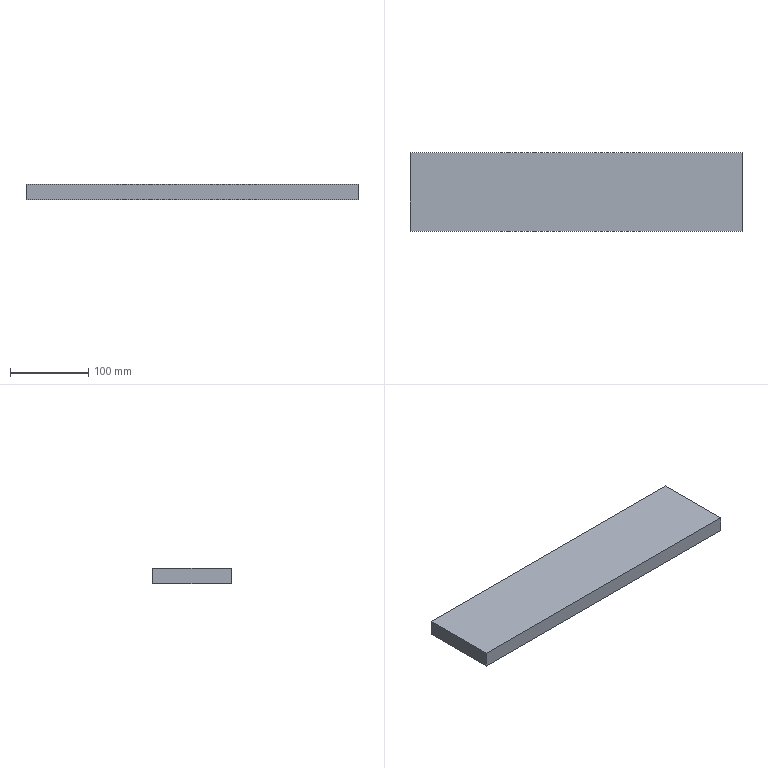Part | SolidWorks | features Extrusion 1 | 1 solid | 6 faces | box 425 x 100 x 20 mm | volume 850000 mm3 | plane 6
STEP:
#1=CARTESIAN_POINT('',(0.,100.,0.));
#2=VERTEX_POINT('',#1);
#3=CARTESIAN_POINT('',(0.,0.,0.));
#4=VERTEX_POINT('',#3);
#5=CARTESIAN_POINT('',(0.,0.,0.));
#6=DIRECTION('',(0.,-1.,0.));
#7=VECTOR('',#6,1000.);
#8=LINE('',#5,#7);
#9=EDGE_CURVE('',#2,#4,#8,.T.);
#10=ORIENTED_EDGE('',*,*,#9,.T.);
#11=CARTESIAN_POINT('',(0.,0.,20.));
#12=VERTEX_POINT('',#11);
#13=CARTESIAN_POINT('',(0.,0.,20.));
#14=DIRECTION('',(0.,0.,-1.));
#15=VECTOR('',#14,1000.);
#16=LINE('',#13,#15);
#17=EDGE_CURVE('',#12,#4,#16,.T.);
#18=ORIENTED_EDGE('',*,*,#17,.F.);
#19=CARTESIAN_POINT('',(0.,100.,20.));
#20=VERTEX_POINT('',#19);
#21=CARTESIAN_POINT('',(0.,0.,20.));
#22=DIRECTION('',(0.,-1.,0.));
#23=VECTOR('',#22,1000.);
#24=LINE('',#21,#23);
#25=EDGE_CURVE('',#20,#12,#24,.T.);
#26=ORIENTED_EDGE('',*,*,#25,.F.);
#27=CARTESIAN_POINT('',(0.,100.,20.));
#28=DIRECTION('',(0.,0.,-1.));
#29=VECTOR('',#28,1000.);
#30=LINE('',#27,#29);
#31=EDGE_CURVE('',#20,#2,#30,.T.);
#32=ORIENTED_EDGE('',*,*,#31,.T.);
#33=EDGE_LOOP('',(#10,#18,#26,#32));
#34=FACE_OUTER_BOUND('',#33,.T.);
#35=CARTESIAN_POINT('',(0.,0.,20.));
#36=DIRECTION('',(1.,0.,0.));
#37=DIRECTION('',(0.,0.,-1.));
#38=AXIS2_PLACEMENT_3D('',#35,#36,#37);
#39=PLANE('',#38);
#40=ADVANCED_FACE('',(#34),#39,.F.);
#41=CARTESIAN_POINT('',(425.,0.,0.));
#42=VERTEX_POINT('',#41);
#43=CARTESIAN_POINT('',(0.,0.,0.));
#44=DIRECTION('',(1.,0.,0.));
#45=VECTOR('',#44,1000.);
#46=LINE('',#43,#45);
#47=EDGE_CURVE('',#4,#42,#46,.T.);
#48=ORIENTED_EDGE('',*,*,#47,.T.);
#49=CARTESIAN_POINT('',(425.,0.,20.));
#50=VERTEX_POINT('',#49);
#51=CARTESIAN_POINT('',(425.,0.,20.));
#52=DIRECTION('',(0.,0.,-1.));
#53=VECTOR('',#52,1000.);
#54=LINE('',#51,#53);
#55=EDGE_CURVE('',#50,#42,#54,.T.);
#56=ORIENTED_EDGE('',*,*,#55,.F.);
#57=CARTESIAN_POINT('',(0.,0.,20.));
#58=DIRECTION('',(1.,0.,0.));
#59=VECTOR('',#58,1000.);
#60=LINE('',#57,#59);
#61=EDGE_CURVE('',#12,#50,#60,.T.);
#62=ORIENTED_EDGE('',*,*,#61,.F.);
#63=ORIENTED_EDGE('',*,*,#17,.T.);
#64=EDGE_LOOP('',(#48,#56,#62,#63));
#65=FACE_OUTER_BOUND('',#64,.T.);
#66=CARTESIAN_POINT('',(0.,0.,20.));
#67=DIRECTION('',(0.,1.,0.));
#68=DIRECTION('',(0.,0.,1.));
#69=AXIS2_PLACEMENT_3D('',#66,#67,#68);
#70=PLANE('',#69);
#71=ADVANCED_FACE('',(#65),#70,.F.);
#72=CARTESIAN_POINT('',(425.,100.,0.));
#73=VERTEX_POINT('',#72);
#74=CARTESIAN_POINT('',(425.,0.,0.));
#75=DIRECTION('',(0.,1.,0.));
#76=VECTOR('',#75,1000.);
#77=LINE('',#74,#76);
#78=EDGE_CURVE('',#42,#73,#77,.T.);
#79=ORIENTED_EDGE('',*,*,#78,.T.);
#80=CARTESIAN_POINT('',(425.,100.,20.));
#81=VERTEX_POINT('',#80);
#82=CARTESIAN_POINT('',(425.,100.,20.));
#83=DIRECTION('',(0.,0.,-1.));
#84=VECTOR('',#83,1000.);
#85=LINE('',#82,#84);
#86=EDGE_CURVE('',#81,#73,#85,.T.);
#87=ORIENTED_EDGE('',*,*,#86,.F.);
#88=CARTESIAN_POINT('',(425.,0.,20.));
#89=DIRECTION('',(0.,1.,0.));
#90=VECTOR('',#89,1000.);
#91=LINE('',#88,#90);
#92=EDGE_CURVE('',#50,#81,#91,.T.);
#93=ORIENTED_EDGE('',*,*,#92,.F.);
#94=ORIENTED_EDGE('',*,*,#55,.T.);
#95=EDGE_LOOP('',(#79,#87,#93,#94));
#96=FACE_OUTER_BOUND('',#95,.T.);
#97=CARTESIAN_POINT('',(425.,0.,20.));
#98=DIRECTION('',(-1.,0.,0.));
#99=DIRECTION('',(0.,0.,1.));
#100=AXIS2_PLACEMENT_3D('',#97,#98,#99);
#101=PLANE('',#100);
#102=ADVANCED_FACE('',(#96),#101,.F.);
#103=CARTESIAN_POINT('',(0.,100.,0.));
#104=DIRECTION('',(-1.,0.,0.));
#105=VECTOR('',#104,1000.);
#106=LINE('',#103,#105);
#107=EDGE_CURVE('',#73,#2,#106,.T.);
#108=ORIENTED_EDGE('',*,*,#107,.T.);
#109=ORIENTED_EDGE('',*,*,#31,.F.);
#110=CARTESIAN_POINT('',(0.,100.,20.));
#111=DIRECTION('',(-1.,0.,0.));
#112=VECTOR('',#111,1000.);
#113=LINE('',#110,#112);
#114=EDGE_CURVE('',#81,#20,#113,.T.);
#115=ORIENTED_EDGE('',*,*,#114,.F.);
#116=ORIENTED_EDGE('',*,*,#86,.T.);
#117=EDGE_LOOP('',(#108,#109,#115,#116));
#118=FACE_OUTER_BOUND('',#117,.T.);
#119=CARTESIAN_POINT('',(0.,100.,20.));
#120=DIRECTION('',(0.,-1.,0.));
#121=DIRECTION('',(0.,0.,-1.));
#122=AXIS2_PLACEMENT_3D('',#119,#120,#121);
#123=PLANE('',#122);
#124=ADVANCED_FACE('',(#118),#123,.F.);
#125=ORIENTED_EDGE('',*,*,#25,.T.);
#126=ORIENTED_EDGE('',*,*,#61,.T.);
#127=ORIENTED_EDGE('',*,*,#92,.T.);
#128=ORIENTED_EDGE('',*,*,#114,.T.);
#129=EDGE_LOOP('',(#125,#126,#127,#128));
#130=FACE_OUTER_BOUND('',#129,.T.);
#131=CARTESIAN_POINT('',(0.,0.,20.));
#132=DIRECTION('',(0.,0.,-1.));
#133=DIRECTION('',(-1.,0.,0.));
#134=AXIS2_PLACEMENT_3D('',#131,#132,#133);
#135=PLANE('',#134);
#136=ADVANCED_FACE('',(#130),#135,.F.);
#137=ORIENTED_EDGE('',*,*,#9,.F.);
#138=ORIENTED_EDGE('',*,*,#107,.F.);
#139=ORIENTED_EDGE('',*,*,#78,.F.);
#140=ORIENTED_EDGE('',*,*,#47,.F.);
#141=EDGE_LOOP('',(#137,#138,#139,#140));
#142=FACE_OUTER_BOUND('',#141,.T.);
#143=CARTESIAN_POINT('',(0.,0.,0.));
#144=DIRECTION('',(0.,0.,-1.));
#145=DIRECTION('',(-1.,0.,0.));
#146=AXIS2_PLACEMENT_3D('',#143,#144,#145);
#147=PLANE('',#146);
#148=ADVANCED_FACE('',(#142),#147,.T.);
#149=CLOSED_SHELL('',(#40,#71,#102,#124,#136,#148));
#150=MANIFOLD_SOLID_BREP('',#149);
#151=CARTESIAN_POINT('',(0.,0.,0.));
#152=DIRECTION('',(0.,0.,1.));
#153=DIRECTION('',(1.,0.,0.));
#154=AXIS2_PLACEMENT_3D('',#151,#152,#153);
#155=(LENGTH_UNIT()NAMED_UNIT(*)SI_UNIT(.MILLI.,.METRE.));
#156=UNCERTAINTY_MEASURE_WITH_UNIT(LENGTH_MEASURE(0.00001),#155,'','');
#157=(NAMED_UNIT(*)PLANE_ANGLE_UNIT()SI_UNIT($,.RADIAN.));
#158=(NAMED_UNIT(*)SI_UNIT($,.STERADIAN.)SOLID_ANGLE_UNIT());
#159=(GEOMETRIC_REPRESENTATION_CONTEXT(3)GLOBAL_UNCERTAINTY_ASSIGNED_CONTEXT((#156))GLOBAL_UNIT_ASSIGNED_CONTEXT((#155,#157,#158))REPRESENTATION_CONTEXT('',''));
#160=ADVANCED_BREP_SHAPE_REPRESENTATION('',(#150,#154),#159);